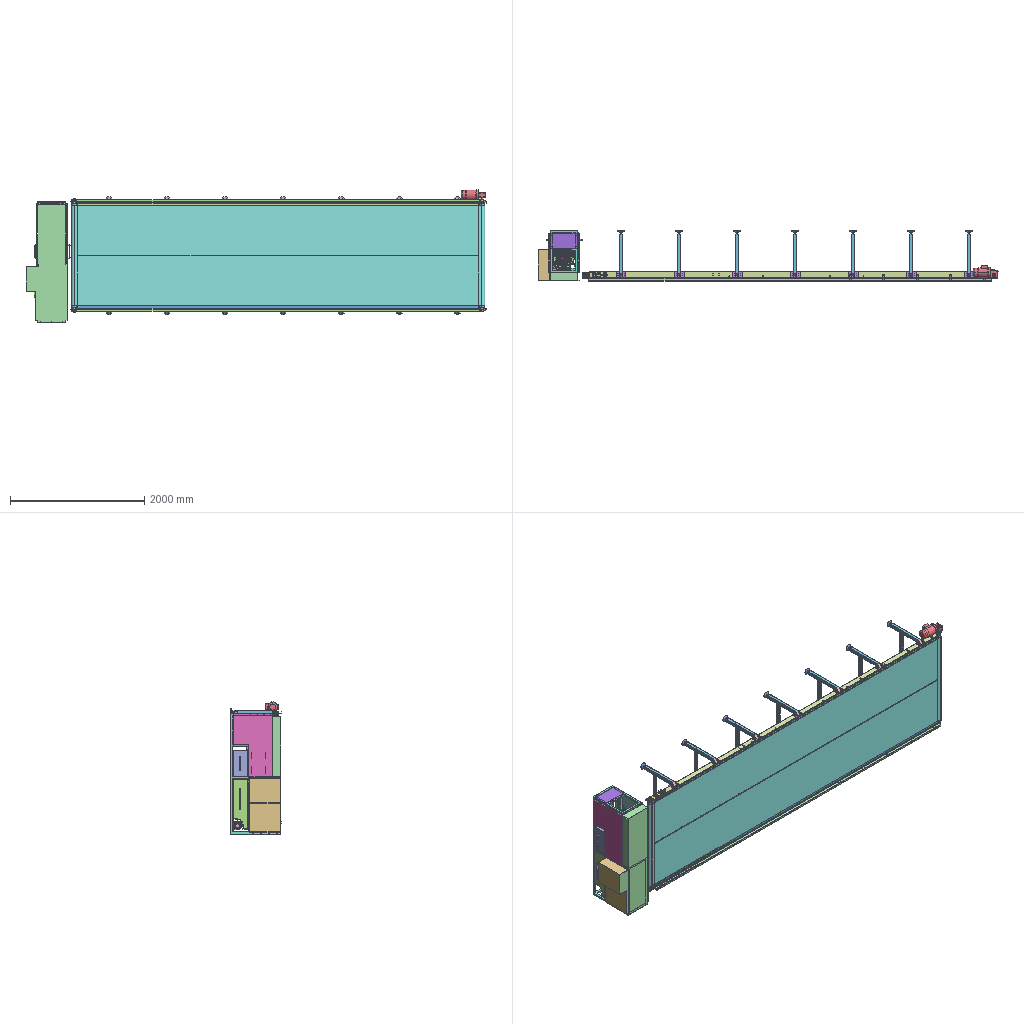Assembly | STEP file | 129 different items | 1049 placed | box 6855 x 752 x 1973 mm
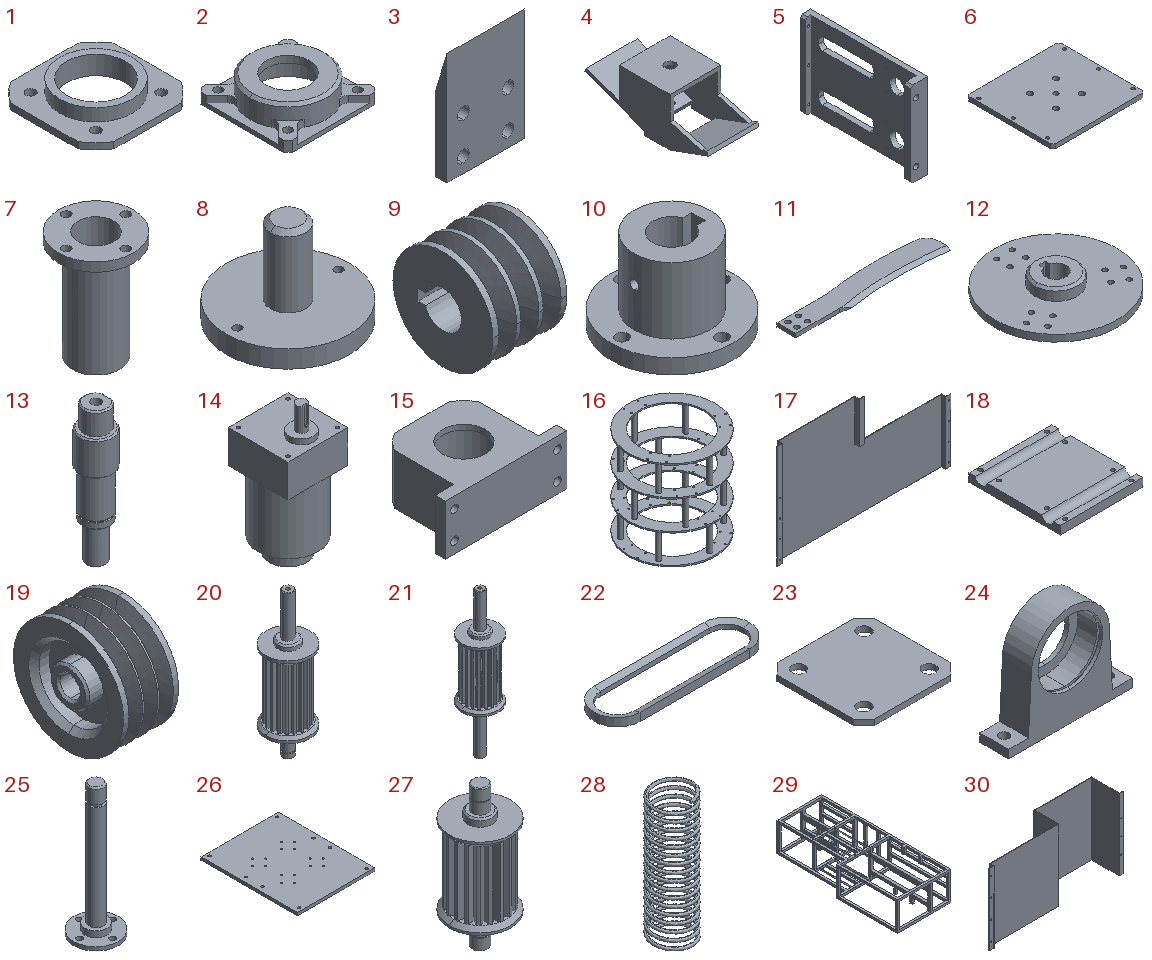Parts list (item | name | quantity | parent item | size | volume):
1 | Bearing cap | x1 | in Cut-off module | 67 x 67 x 12 mm | 16840 mm3
2 | Bearing seat | x8 | in Conveyor mechanism | 68 x 68 x 19 mm | 28550 mm3
3 | Blade | x12 | in Tool holder assembly | 20.7 x 3 x 30 mm | 1456 mm3
4 | Blade fixing bracket | x12 | in Tool holder assembly | 40 x 96.985 x 38 mm | 22805 mm3
5 | Bracket | x4 | in Conveyor mechanism | 40 x 275 x 200 mm | 655765 mm3
6 | Bracket upper plate | x2 | in Conveyor mechanism | 214 x 200 x 10 mm | 419850 mm3
7 | Bushing | x12 | in Tool holder assembly | 25 x 25 x 36 mm | 3962 mm3
8 | Clamping screw | x1 | in Cut-off module | 28 x 28 x 20 mm | 3235 mm3
9 | Constant-speed small pulley | x4 | in Conveyor mechanism | 40 x 54 x 54 mm | 49564 mm3
10 | Coupling | x2 | in Cut-off module | 45 x 45 x 30 mm | 18366 mm3
11 | Cut-off blade | x3 | in Cut-off module | 200 x 35.06 x 5 mm | 25538 mm3
12 | Cut-off cutter head | x1 | in Cut-off module | 110 x 110 x 16 mm | 62709 mm3
13 | Cut-off drive shaft | x1 | in Cut-off module | 24 x 24 x 101 mm | 28813 mm3
14 | Cut-off geared motor | x1 | in Cut-off module | 80 x 80 x 182 mm | 732361 mm3
15 | Cut-off module bearing seat | x1 | in Cut-off module | 97 x 67 x 40 mm | 117140 mm3
16 | Cutter head | x1 | in Cutter head assembly | 310 x 310 x 320 mm | 992722 mm3
17 | Cutting guard | x1 | in Assembly | 970 x 28 x 580 mm | 1440851 mm3
18 | Cutting module fixing bracket | x16 | in Cutter head assembly | 100 x 110 x 10 mm | 96984 mm3
19 | Driven pulley | x2 | in Conveyor mechanism | 54 x 108 x 108 mm | 283345 mm3
20 | Driven roller | x2 | in Conveyor mechanism | 85 x 85 x 282 mm | 574522 mm3
21 | Driving roller | x2 | in Conveyor mechanism | 85 x 85 x 342 mm | 592269 mm3
22 | Flat belt | x2 | in Assembly | 156 x 46 x 8 mm | 12857 mm3
23 | Floating adjusting plate | x2 | in Conveyor mechanism | 90 x 90 x 5 mm | 37238 mm3
24 | Floating bearing seat | x8 | in Conveyor mechanism | 90 x 21 x 73.5 mm | 51674 mm3
25 | Floating guide shaft | x8 | in Conveyor mechanism | 36 x 36 x 107 mm | 15245 mm3
26 | Floating plate | x2 | in Conveyor mechanism | 161 x 200 x 6 mm | 191436 mm3
27 | Floating roller | x4 | in Conveyor mechanism | 80 x 80 x 185 mm | 409392 mm3
28 | Floating spring | x8 | in Conveyor mechanism | 16.2 x 16.2 x 52 mm | 929.653 mm3
29 | Frame | x1 | in Assembly | 740 x 1790 x 402.356 mm | 20261425 mm3
30 | Guard 4 | x1 | in Assembly | 845 x 178 x 450 mm | 1612656 mm3
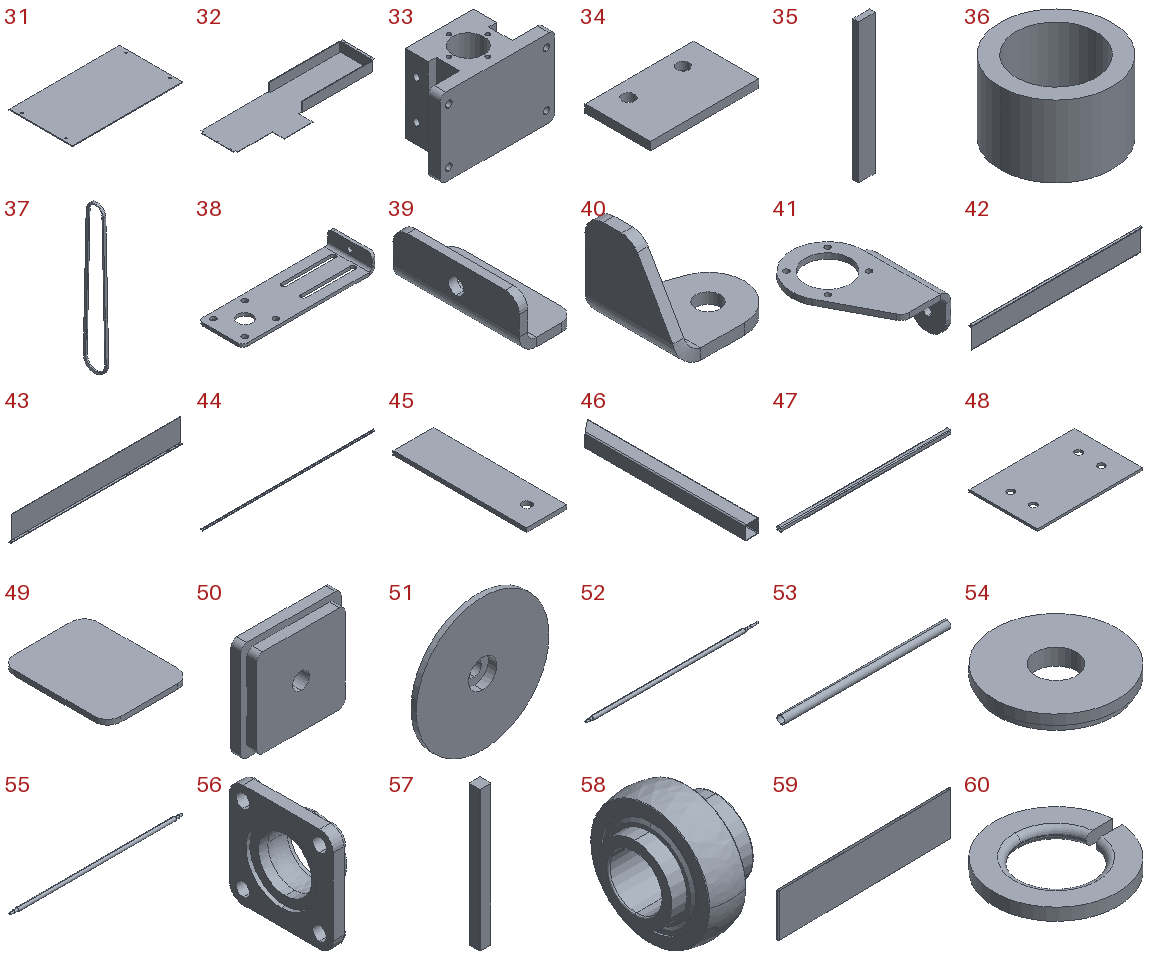31 | Guard 7 | x1 | in Assembly | 402 x 230 x 3 mm | 277041 mm3
32 | Guard 8 | x1 | in Assembly | 1787 x 612 x 124 mm | 4313397 mm3
33 | Guide fixing seat | x12 | in Tool holder assembly | 59 x 30 x 40 mm | 35183 mm3
34 | Guide pressure plate | x24 | in Tool holder assembly | 40 x 24 x 3 mm | 2785 mm3
35 | Guide strip | x24 | in Tool holder assembly | 12 x 4 x 100 mm | 4800 mm3
36 | Large pulley shaft collar | x2 | in Conveyor mechanism | 28 x 28 x 18 mm | 5429 mm3
37 | Long V-belt | x1 | in Assembly | 11 x 98 x 629.5 mm | 91301 mm3
38 | Microwave Drying Flat Conveyor-CN2500x400-101-101 | x2 | in Microwave Drying Flat Conveyor-CN2500x400-101-100 | 270 x 90 x 36 mm | 137966 mm3
39 | Microwave Drying Flat Conveyor-CN2500x400-101-102 | x2 | in Microwave Drying Flat Conveyor-CN2500x400-101-100 | 40 x 90 x 36 mm | 33488 mm3
40 | Microwave Drying Flat Conveyor-CN2500x400-102-101 | x1 | in Microwave Drying Flat Conveyor-CN2500x400-102-100 | 56 x 52 x 51 mm | 22223 mm3
41 | Microwave Drying Flat Conveyor-CN2500x400-102-102 | x1 | in Microwave Drying Flat Conveyor-CN2500x400-102-100 | 92 x 125 x 49 mm | 51756 mm3
42 | Microwave Drying Flat Conveyor-CN2500x400-103-101a | x1 | in 微波烘干-平输送机构-Assembly 2 | 6084 x 93 x 803 mm | 16530711 mm3
43 | Microwave Drying Flat Conveyor-CN2500x400-103-101b | x1 | in 微波烘干-平输送机构-Assembly 2 | 6084 x 100 x 803 mm | 16658166 mm3
44 | Microwave Drying Flat Conveyor-CN2500x400-104-101_DefaultSM-FLAT-PATTERN | x2 | in Microwave Drying Flat Conveyor-CN2500x400-104a-100, Microwave Drying Flat Conveyor-CN2500x400-104b-100 | 6000 x 50 x 47 mm | 1622469 mm3
45 | Microwave Drying Flat Conveyor-CN2500x400-104-102 | x10 | in Microwave Drying Flat Conveyor-CN2500x400-104a-100, Microwave Drying Flat Conveyor-CN2500x400-104b-100 | 30 x 100 x 3 mm | 8885 mm3
46 | Microwave Drying Flat Conveyor-CN2500x400-105-101_Default<Machining blank> | x14 | in Microwave Drying Flat Conveyor-CN2500x400-105-100 | 50 x 620 x 50 mm | 224219 mm3
47 | Microwave Drying Flat Conveyor-CN2500x400-105-102_Default<Machining blank> | x7 | in Microwave Drying Flat Conveyor-CN2500x400-105-100 | 1612 x 40 x 40 mm | 862092 mm3
48 | Microwave Drying Flat Conveyor-CN2500x400-105-103 | x14 | in Microwave Drying Flat Conveyor-CN2500x400-105-100 | 140 x 90 x 3 mm | 37037 mm3
49 | Microwave Drying Flat Conveyor-CN2500x400-105-104 | x14 | in Microwave Drying Flat Conveyor-CN2500x400-105-100 | 50 x 64 x 3 mm | 9435 mm3
50 | Microwave Drying Flat Conveyor-CN2500x400-105-105 | x14 | in Microwave Drying Flat Conveyor-CN2500x400-105-100 | 50 x 10 x 50 mm | 21535 mm3
51 | Microwave Drying Flat Conveyor-CN2500x400-105-106 | x14 | in 51 | 100 x 20 x 100 mm | 96687 mm3
52 | Microwave Drying Flat Conveyor-CN2500x400-107-101 | x1 | in Microwave Drying Flat Conveyor-CN2500x400-107-100 | 1746 x 35 x 35 mm | 1552118 mm3
53 | Microwave Drying Flat Conveyor-CN2500x400-107-102 | x2 | in Microwave Drying Flat Conveyor-CN2500x400-107-100, Microwave Drying Flat Conveyor-CN2500x400-108-100 | 1550 x 75 x 75 mm | 710942 mm3
54 | Microwave Drying Flat Conveyor-CN2500x400-107-103 | x4 | in Microwave Drying Flat Conveyor-CN2500x400-107-100, Microwave Drying Flat Conveyor-CN2500x400-108-100 | 75 x 75 x 10 mm | 37435 mm3
55 | Microwave Drying Flat Conveyor-CN2500x400-108-101 | x1 | in Microwave Drying Flat Conveyor-CN2500x400-108-100 | 1682 x 35 x 35 mm | 1539685 mm3
56 | Microwave Drying Flat Conveyor-FY 504 U_VA228_fyva_Default | x2 | in Microwave Drying Flat Conveyor-FY 20 TF_VA228_Default | 29.5 x 86 x 86 mm | 59887 mm3
57 | Microwave Drying Flat Conveyor-Key 6x6x70 | x1 | in 微波烘干-平输送机构-Assembly 2 | 6 x 6 x 75 mm | 2686 mm3
58 | Microwave Drying Flat Conveyor-YAR 204-2FW_VA228_Default | x2 | in Microwave Drying Flat Conveyor-FY 20 TF_VA228_Default | 31 x 47 x 47 mm | 24116 mm3
59 | Microwave Drying Flat Conveyor-dai | x1 | in 微波烘干-平输送机构-Assembly 2 | 6157 x 175.545 x 1500 mm | 52078468 mm3
60 | Microwave Drying Flat Conveyor-din_128_a12 | x12 | in Microwave Drying Flat Conveyor-CN2500x400-101-100 | 21.067 x 21.1 x 2.1 mm | 456.756 mm3
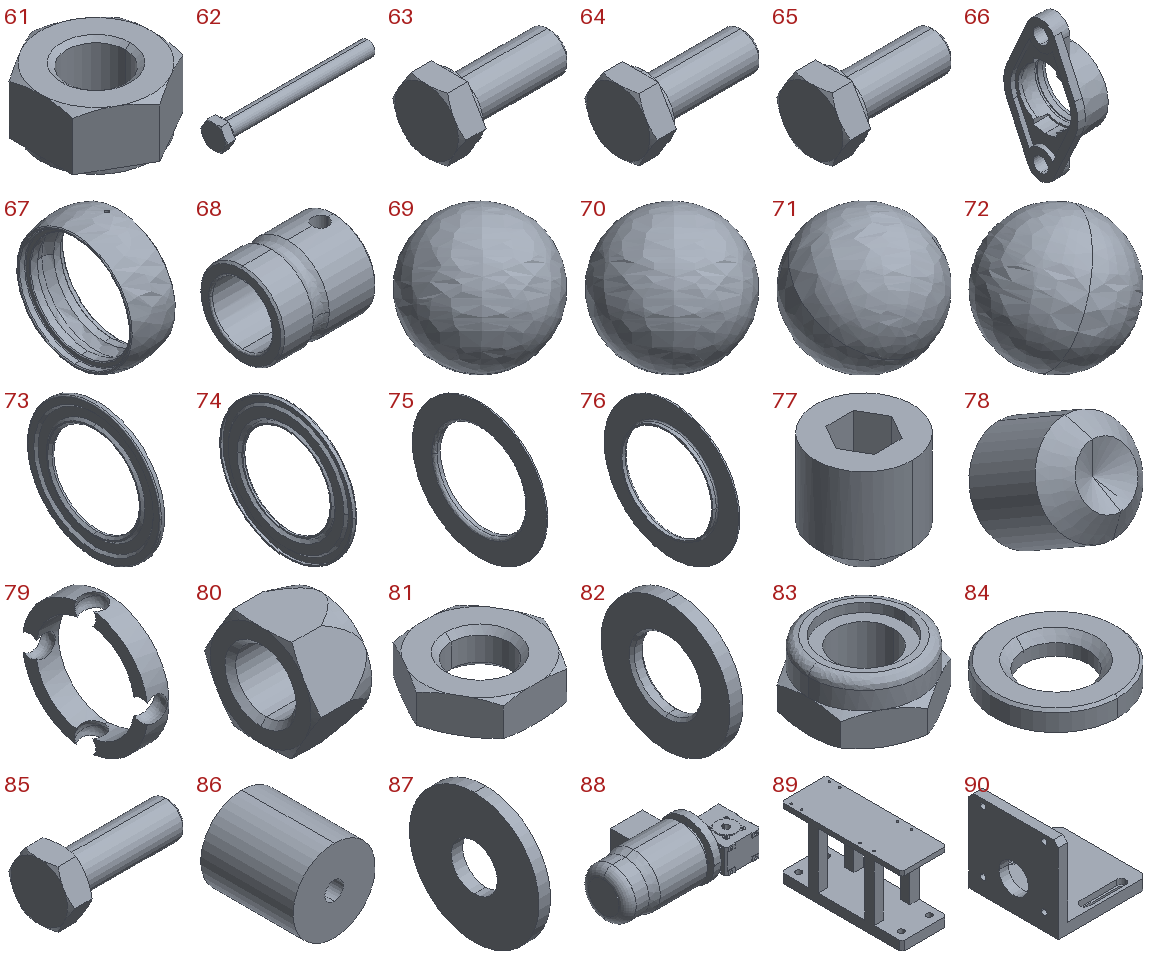61 | Microwave Drying Flat Conveyor-hex nut style 1 gradeab_din_Hexagon Nut ISO 4032 - M10 - W - N_Default | x14 | in 51 | 16 x 18.475 x 8.4 mm | 1357 mm3
62 | Microwave Drying Flat Conveyor-hex screw gradeab_din_DIN EN 24017 - M10 x 100-N_Default | x16 | in Microwave Drying Flat Conveyor-CN2500x400-101-100, 51 | 106.4 x 18.475 x 16 mm | 9247 mm3
63 | Microwave Drying Flat Conveyor-hex screw gradeab_din_DIN EN 24017 - M10 x 25-N_Default | x2 | in 微波烘干-平输送机构-Assembly 2 | 31.4 x 18.475 x 16 mm | 3356 mm3
64 | Microwave Drying Flat Conveyor-hex screw gradeab_din_DIN EN 24017 - M6 x 16-N_Default | x11 | in 微波烘干-平输送机构-Assembly 2 | 20 x 11.547 x 10 mm | 791.21 mm3
65 | Microwave Drying Flat Conveyor-hex screw gradeab_din_DIN EN 24017 - M8 x 20-N_Default | x2 | in Microwave Drying Flat Conveyor-CN2500x400-102-100 | 25.3 x 15.011 x 13 mm | 1766 mm3
66 | Microwave Drying Flat Conveyor-inafag_ucfl204_62o9y6gnj3059x015y4y3bh4_01 | x2 | in Microwave Drying Flat Conveyor-inafag_ucfl204_62o9y6gnj3059x015y4y3bh4 | - | -
67 | Microwave Drying Flat Conveyor-inafag_ucfl204_62o9y6gnj3059x015y4y3bh4_02 | x2 | in Microwave Drying Flat Conveyor-inafag_ucfl204_62o9y6gnj3059x015y4y3bh4 | 17 x 47.603 x 47 mm | 6473 mm3
68 | Microwave Drying Flat Conveyor-inafag_ucfl204_62o9y6gnj3059x015y4y3bh4_03 | x2 | in Microwave Drying Flat Conveyor-inafag_ucfl204_62o9y6gnj3059x015y4y3bh4 | 31 x 27.56 x 27.56 mm | 8243 mm3
69 | Microwave Drying Flat Conveyor-inafag_ucfl204_62o9y6gnj3059x015y4y3bh4_04 | x2 | in Microwave Drying Flat Conveyor-inafag_ucfl204_62o9y6gnj3059x015y4y3bh4 | 7.94 x 7.94 x 7.94 mm | 262.089 mm3
70 | Microwave Drying Flat Conveyor-inafag_ucfl204_62o9y6gnj3059x015y4y3bh4_05 | x2 | in Microwave Drying Flat Conveyor-inafag_ucfl204_62o9y6gnj3059x015y4y3bh4 | 7.94 x 7.94 x 7.94 mm | 262.089 mm3
71 | Microwave Drying Flat Conveyor-inafag_ucfl204_62o9y6gnj3059x015y4y3bh4_06 | x2 | in Microwave Drying Flat Conveyor-inafag_ucfl204_62o9y6gnj3059x015y4y3bh4 | 7.94 x 7.94 x 7.94 mm | 262.089 mm3
72 | Microwave Drying Flat Conveyor-inafag_ucfl204_62o9y6gnj3059x015y4y3bh4_07 | x2 | in Microwave Drying Flat Conveyor-inafag_ucfl204_62o9y6gnj3059x015y4y3bh4 | 7.94 x 7.94 x 7.94 mm | 262.089 mm3
73 | Microwave Drying Flat Conveyor-inafag_ucfl204_62o9y6gnj3059x015y4y3bh4_08 | x2 | in Microwave Drying Flat Conveyor-inafag_ucfl204_62o9y6gnj3059x015y4y3bh4 | 1.397 x 42 x 42 mm | 599.425 mm3
74 | Microwave Drying Flat Conveyor-inafag_ucfl204_62o9y6gnj3059x015y4y3bh4_09 | x2 | in Microwave Drying Flat Conveyor-inafag_ucfl204_62o9y6gnj3059x015y4y3bh4 | 1.397 x 42 x 42 mm | 599.533 mm3
75 | Microwave Drying Flat Conveyor-inafag_ucfl204_62o9y6gnj3059x015y4y3bh4_10 | x2 | in Microwave Drying Flat Conveyor-inafag_ucfl204_62o9y6gnj3059x015y4y3bh4 | 1.812 x 41.16 x 41.16 mm | 343.087 mm3
76 | Microwave Drying Flat Conveyor-inafag_ucfl204_62o9y6gnj3059x015y4y3bh4_11 | x2 | in Microwave Drying Flat Conveyor-inafag_ucfl204_62o9y6gnj3059x015y4y3bh4 | 1.812 x 41.16 x 41.16 mm | 343.35 mm3
77 | Microwave Drying Flat Conveyor-inafag_ucfl204_62o9y6gnj3059x015y4y3bh4_12 | x2 | in Microwave Drying Flat Conveyor-inafag_ucfl204_62o9y6gnj3059x015y4y3bh4 | 6 x 6 x 6 mm | 135.214 mm3
78 | Microwave Drying Flat Conveyor-inafag_ucfl204_62o9y6gnj3059x015y4y3bh4_13 | x2 | in Microwave Drying Flat Conveyor-inafag_ucfl204_62o9y6gnj3059x015y4y3bh4 | 6 x 7.571 x 7.571 mm | 135.214 mm3
79 | Microwave Drying Flat Conveyor-inafag_ucfl204_62o9y6gnj3059x015y4y3bh4_14 | x2 | in Microwave Drying Flat Conveyor-inafag_ucfl204_62o9y6gnj3059x015y4y3bh4 | - | 2155 mm3
80 | Microwave Drying Flat Conveyor-nut_gb_t_6185_1_m6 | x10 | in 微波烘干-平输送机构-Assembly 2 | 6 x 11.547 x 10 mm | 336.581 mm3
81 | Microwave Drying Flat Conveyor-nut_iso_4035_-_d_m10_-_05 | x32 | in Microwave Drying Flat Conveyor-CN2500x400-101-100 | 18.475 x 16 x 5 mm | 809.954 mm3
82 | Microwave Drying Flat Conveyor-plain washer hardened grade a_din_Washer DIN 125 - A 10.5 - 300HV_Default | x4 | in 微波烘干-平输送机构-Assembly 2 | 2 x 20 x 20 mm | 449.726 mm3
83 | Microwave Drying Flat Conveyor-prevailing torque nut thin insert_din_DIN EN ISO 10511 - M10 - N_Default | x2 | in 微波烘干-平输送机构-Assembly 2 | 16 x 18.475 x 8.56 mm | 1235 mm3
84 | Microwave Drying Flat Conveyor-rondelle_iso_7416-12 | x40 | in Microwave Drying Flat Conveyor-CN2500x400-101-100 | 25 x 25 x 4 mm | 1366 mm3
85 | Microwave Drying Flat Conveyor-screw_gb_t_6563_m10x30 | x20 | in Microwave Drying Flat Conveyor-CN2500x400-101-100 | 36.4 x 18.475 x 16 mm | 3756 mm3
86 | Microwave Drying Flat Conveyor-silenbloc 40x45xm8 | x1 | in Microwave Drying Flat Conveyor-CN2500x400-102-100 | 40 x 45 x 40 mm | 54907 mm3
87 | Microwave Drying Flat Conveyor-washer_gb_t_96_1_6 | x6 | in 微波烘干-平输送机构-Assembly 2 | 1.6 x 18 x 18 mm | 355.679 mm3
88 | Microwave Drying Flat Conveyor-worm gear reducer_mu40-base-10-b3 | x1 | in 微波烘干-平输送机构-Assembly 2 | 361 x 200 x 160 mm | 5383182 mm3
89 | Motor bracket | x1 | in Cut-off module | 97 x 260 x 150 mm | 936866 mm3
90 | Motor fixing bracket | x1 | in Cut-off module | 97 x 97 x 91.5 mm | 167399 mm3
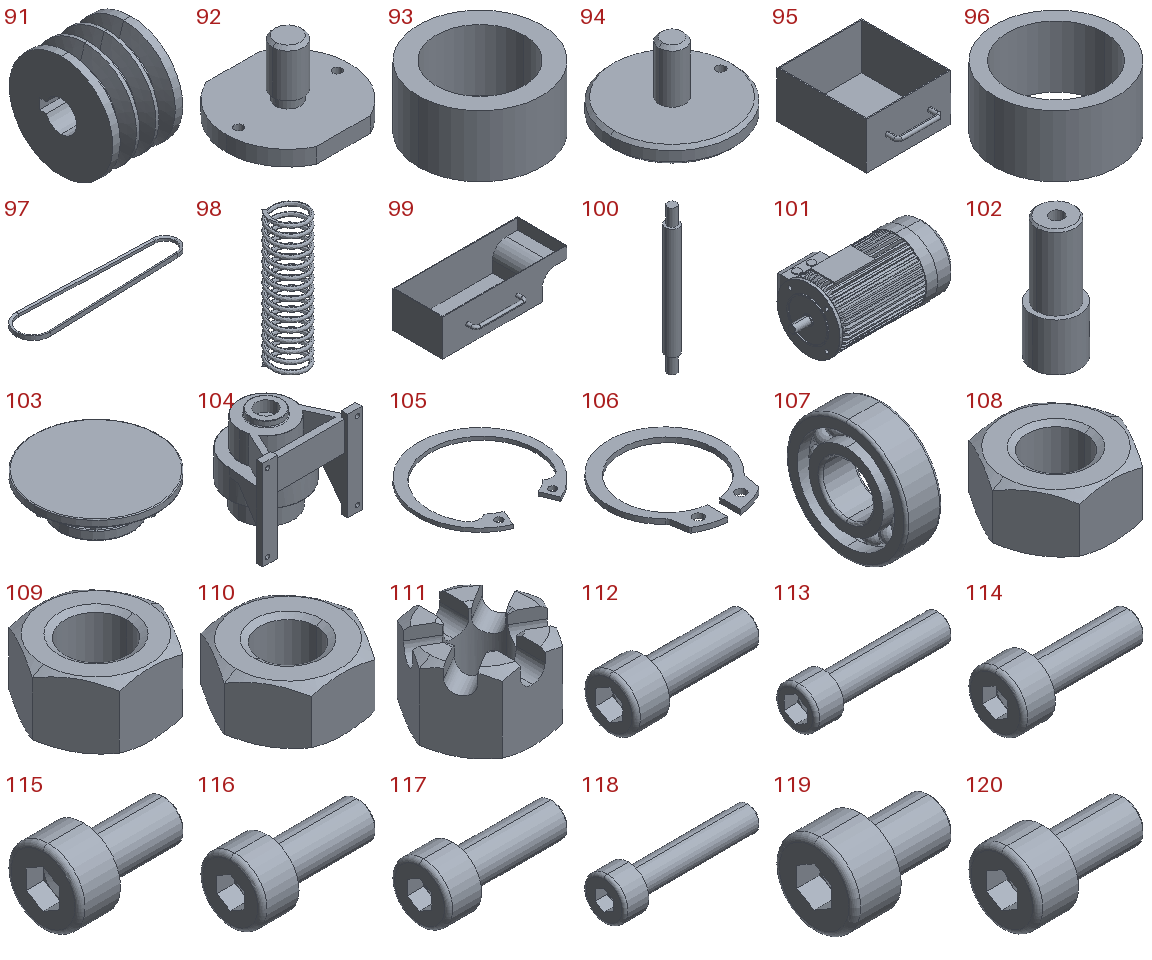91 | Motor pulley | x2 | in Belt drive motor | 54 x 80 x 80 mm | 176576 mm3
92 | Motor pulley screw | x2 | in Belt drive motor | 40 x 36 x 23 mm | 7301 mm3
93 | Pulley end bushing | x4 | in Conveyor mechanism | 28 x 28 x 14 mm | 4222 mm3
94 | Pulley locating pin | x6 | in Conveyor mechanism | 38 x 38 x 21 mm | 6315 mm3
95 | Scrap collection box | x1 | in Assembly | 400 x 540 x 220 mm | 2744863 mm3
96 | Shaft collar | x8 | in Conveyor mechanism | 28 x 28 x 14 mm | 3299 mm3
97 | Short V-belt | x1 | in Assembly | 446 x 94 x 11 mm | 53257 mm3
98 | Spring | x12 | in Tool holder assembly | 15.5 x 15.5 x 57 mm | 1160 mm3
99 | Sugarcane segment collection box | x1 | in Assembly | 750 x 360 x 220 mm | 3249841 mm3
100 | Tool bar | x12 | in Tool holder assembly | 12 x 12 x 130 mm | 12818 mm3
101 | XB motor_BWED3922_Y_90L.step | x2 | in Belt drive motor | 170 x 100 x 80 mm | 524575 mm3
102 | XB output shaft_100_165_28.step | x2 | in Belt drive motor | 30 x 30 x 76.8 mm | 41146 mm3
103 | XB-Connecting flange_BWED3922_90B5.step | x2 | in Belt drive motor | 122.4 x 122.4 x 36.36 mm | 150900 mm3
104 | XWE main body_BWED3922.step | x2 | in Belt drive motor | 148.8 x 124.8 x 134.4 mm | 938232 mm3
105 | circlips for hole--type b gb_GB_CONNECTING_PIECE_RINGS_CHB 47 | x8 | in Conveyor mechanism | 50.5 x 48.578 x 1.5 mm | 798.879 mm3
106 | circlips for shaft--type a large gb_GB_CONNECTING_PIECE_RING_RRA 20 | x12 | in Conveyor mechanism | 22.5 x 25.161 x 1 mm | 153.893 mm3
107 | deep groove ball bearings gb_Rolling bearings 6204 GB 276-94 | x18 | in Conveyor mechanism, Cut-off module | 14 x 47 x 47 mm | 14611 mm3
108 | hex nuts, style 1-grades ab gb_GB_FASTENER_NUT_SNAB1 M10-N | x8 | in Conveyor mechanism | 18.475 x 16 x 8.4 mm | 1367 mm3
109 | hex nuts, style 1-grades ab gb_GB_FASTENER_NUT_SNAB1 M12-N | x2 | in Conveyor mechanism | 20.785 x 18 x 10.8 mm | 2118 mm3
110 | hex nuts, style 1-grades ab gb_GB_FASTENER_NUT_SNAB1 M8-N | x12 | in Tool holder assembly | 15.011 x 13 x 6.8 mm | 739.531 mm3
111 | hex slotted and castle nuts 1-grade ab gb_GB_FASTENER_NUT_SNNAB1 M8 YB-N | x12 | in Tool holder assembly | 15.011 x 13 x 9.8 mm | 915.149 mm3
112 | hexagon socket head cap screws gb_GB_FASTENER_SCREWS_HSHCS M10X30-N | x12 | in Assembly | 40 x 16 x 16 mm | 4032 mm3
113 | hexagon socket head cap screws gb_GB_FASTENER_SCREWS_HSHCS M12X50-N | x2 | in Conveyor mechanism | 62 x 18 x 18 mm | 8080 mm3
114 | hexagon socket head cap screws gb_GB_FASTENER_SCREWS_HSHCS M2.5X8-N | x48 | in Tool holder assembly | 10.5 x 4.5 x 4.5 mm | 74.29 mm3
115 | hexagon socket head cap screws gb_GB_FASTENER_SCREWS_HSHCS M3X6-N | x48 | in Tool holder assembly | 9 x 5.5 x 5.5 mm | 104.917 mm3
116 | hexagon socket head cap screws gb_GB_FASTENER_SCREWS_HSHCS M4X10-N | x48 | in Cutter head assembly | 14 x 7 x 7 mm | 260.588 mm3
117 | hexagon socket head cap screws gb_GB_FASTENER_SCREWS_HSHCS M4X12-N | x4 | in Cut-off module | 16 x 7 x 7 mm | 285.72 mm3
118 | hexagon socket head cap screws gb_GB_FASTENER_SCREWS_HSHCS M4X20-N | x63 | in Cutter head assembly | 24 x 7 x 7 mm | 386.251 mm3
119 | hexagon socket head cap screws gb_GB_FASTENER_SCREWS_HSHCS M4X6-N | x32 | in Conveyor mechanism | 10 x 7 x 7 mm | 210.322 mm3
120 | hexagon socket head cap screws gb_GB_FASTENER_SCREWS_HSHCS M4X8-N | x48 | in Tool holder assembly | 12 x 7 x 7 mm | 235.455 mm3
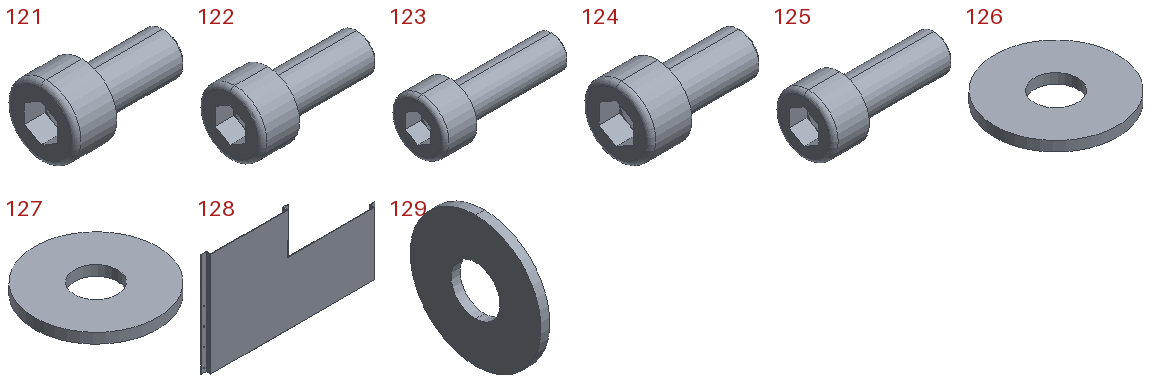121 | hexagon socket head cap screws gb_GB_FASTENER_SCREWS_HSHCS M5X10-N | x12 | in Cut-off module | 15 x 8.5 x 8.5 mm | 438.126 mm3
122 | hexagon socket head cap screws gb_GB_FASTENER_SCREWS_HSHCS M5X12-N | x12 | in Cut-off module | 17 x 8.5 x 8.5 mm | 477.396 mm3
123 | hexagon socket head cap screws gb_GB_FASTENER_SCREWS_HSHCS M5X16-N | x36 | in Conveyor mechanism, Cut-off module | 21 x 8.5 x 8.5 mm | 555.936 mm3
124 | hexagon socket head cap screws gb_GB_FASTENER_SCREWS_HSHCS M6X12-N | x16 | in Conveyor mechanism | 18 x 10 x 10 mm | 731.894 mm3
125 | hexagon socket head cap screws gb_GB_FASTENER_SCREWS_HSHCS M6X16-N | x12 | in Conveyor mechanism | 22 x 10 x 10 mm | 844.992 mm3
126 | plain washers-l series-grades ac gb_GB_FASTENER_WASHER_PWLAC 12 | x8 | in Conveyor mechanism | 37 x 37 x 3 mm | 2827 mm3
127 | plain washers-l series-grades ac gb_GB_FASTENER_WASHER_PWLAC 8 | x12 | in Tool holder assembly | 24 x 24 x 2 mm | 793.943 mm3
128 | 切削Guard 2 | x1 | in Assembly | 970 x 28 x 580 mm | 1440851 mm3
129 | 微波烘干-平输送机构-625058 | x2 | in Microwave Drying Flat Conveyor-CN2500x400-102-100 | 1.5 x 22 x 22 mm | 490.015 mm3